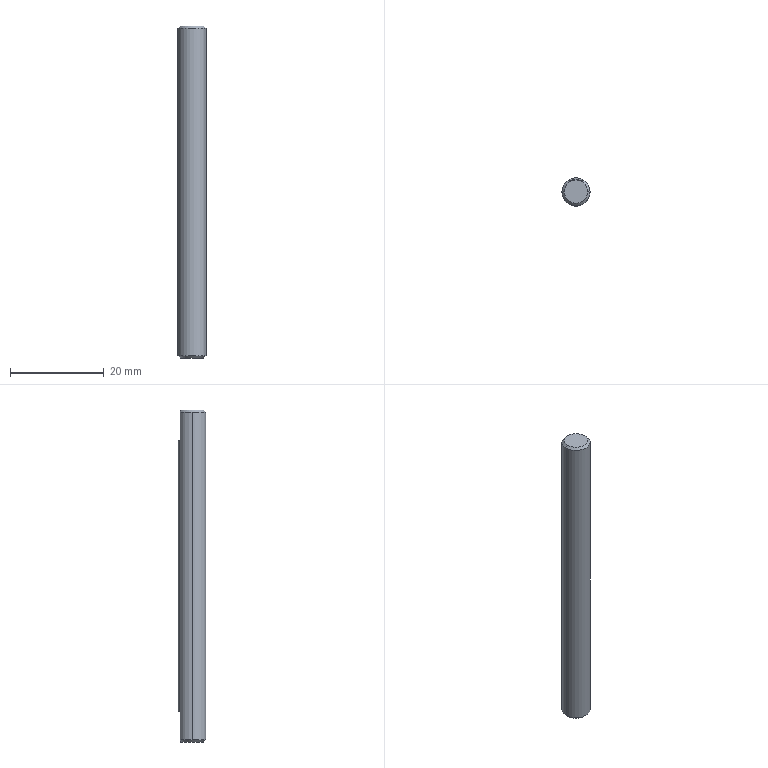Part | STEP file | 10000020485swp000-1 | 1 solid | 14 faces | box 6 x 6 x 71 mm | volume 1989 mm3 | cone 6 | plane 6 | cylinder 2 | commonest cylinder face diameters 6 x2
STEP:
#1=CARTESIAN_POINT('',(2.5,0.,0.));
#2=VERTEX_POINT('',#1);
#3=CARTESIAN_POINT('',(0.,2.5,0.));
#4=VERTEX_POINT('',#3);
#5=CARTESIAN_POINT('',(0.,0.,0.));
#6=DIRECTION('',(0.,0.,1.));
#7=DIRECTION('',(1.,0.,0.));
#8=AXIS2_PLACEMENT_3D('',#5,#6,#7);
#9=CIRCLE('',#8,2.5);
#10=EDGE_CURVE('',#2,#4,#9,.T.);
#11=ORIENTED_EDGE('',*,*,#10,.F.);
#12=CARTESIAN_POINT('',(3.,0.,-0.5));
#13=VERTEX_POINT('',#12);
#14=CARTESIAN_POINT('',(2.5,0.,0.));
#15=DIRECTION('',(0.7071,0.,-0.7071));
#16=VECTOR('',#15,1000.);
#17=LINE('',#14,#16);
#18=EDGE_CURVE('',#2,#13,#17,.T.);
#19=ORIENTED_EDGE('',*,*,#18,.T.);
#20=CARTESIAN_POINT('',(1.658,2.5,-0.5));
#21=VERTEX_POINT('',#20);
#22=CARTESIAN_POINT('',(0.,0.,-0.5));
#23=DIRECTION('',(0.,0.,-1.));
#24=DIRECTION('',(1.,0.,0.));
#25=AXIS2_PLACEMENT_3D('',#22,#23,#24);
#26=CIRCLE('',#25,3.);
#27=EDGE_CURVE('',#21,#13,#26,.T.);
#28=ORIENTED_EDGE('',*,*,#27,.F.);
#29=CARTESIAN_POINT('',(0.,2.5,0.));
#30=CARTESIAN_POINT('',(0.294,2.5,0.));
#31=CARTESIAN_POINT('',(0.5798,2.5,-0.05267));
#32=CARTESIAN_POINT('',(1.139,2.5,-0.2346));
#33=CARTESIAN_POINT('',(1.404,2.5,-0.3596));
#34=CARTESIAN_POINT('',(1.658,2.5,-0.5));
#35=B_SPLINE_CURVE_WITH_KNOTS('',3,(#29,#30,#31,#32,#33,#34),.UNSPECIFIED.,.F.,.F.,(4,2,4),(0.003858,0.004729,0.005601),.UNSPECIFIED.);
#36=EDGE_CURVE('',#4,#21,#35,.T.);
#37=ORIENTED_EDGE('',*,*,#36,.F.);
#38=EDGE_LOOP('',(#11,#19,#28,#37));
#39=FACE_OUTER_BOUND('',#38,.T.);
#40=CARTESIAN_POINT('',(0.,0.,0.));
#41=DIRECTION('',(0.,0.,-1.));
#42=DIRECTION('',(-1.,0.,0.));
#43=AXIS2_PLACEMENT_3D('',#40,#41,#42);
#44=CONICAL_SURFACE('',#43,2.5,0.7854);
#45=ADVANCED_FACE('',(#39),#44,.T.);
#46=ORIENTED_EDGE('',*,*,#18,.F.);
#47=CARTESIAN_POINT('',(-2.5,0.,0.));
#48=VERTEX_POINT('',#47);
#49=CARTESIAN_POINT('',(0.,0.,0.));
#50=DIRECTION('',(0.,0.,1.));
#51=DIRECTION('',(1.,0.,0.));
#52=AXIS2_PLACEMENT_3D('',#49,#50,#51);
#53=CIRCLE('',#52,2.5);
#54=EDGE_CURVE('',#48,#2,#53,.T.);
#55=ORIENTED_EDGE('',*,*,#54,.F.);
#56=CARTESIAN_POINT('',(-3.,0.,-0.5));
#57=VERTEX_POINT('',#56);
#58=CARTESIAN_POINT('',(-2.5,0.,0.));
#59=DIRECTION('',(-0.7071,0.,-0.7071));
#60=VECTOR('',#59,1000.);
#61=LINE('',#58,#60);
#62=EDGE_CURVE('',#48,#57,#61,.T.);
#63=ORIENTED_EDGE('',*,*,#62,.T.);
#64=CARTESIAN_POINT('',(0.,0.,-0.5));
#65=DIRECTION('',(0.,0.,-1.));
#66=DIRECTION('',(1.,0.,0.));
#67=AXIS2_PLACEMENT_3D('',#64,#65,#66);
#68=CIRCLE('',#67,3.);
#69=EDGE_CURVE('',#13,#57,#68,.T.);
#70=ORIENTED_EDGE('',*,*,#69,.F.);
#71=EDGE_LOOP('',(#46,#55,#63,#70));
#72=FACE_OUTER_BOUND('',#71,.T.);
#73=CARTESIAN_POINT('',(0.,0.,0.));
#74=DIRECTION('',(0.,0.,-1.));
#75=DIRECTION('',(-1.,0.,0.));
#76=AXIS2_PLACEMENT_3D('',#73,#74,#75);
#77=CONICAL_SURFACE('',#76,2.5,0.7854);
#78=ADVANCED_FACE('',(#72),#77,.T.);
#79=CARTESIAN_POINT('',(-2.5,0.,-71.));
#80=VERTEX_POINT('',#79);
#81=CARTESIAN_POINT('',(0.,2.5,-71.));
#82=VERTEX_POINT('',#81);
#83=CARTESIAN_POINT('',(0.,0.,-71.));
#84=DIRECTION('',(0.,0.,-1.));
#85=DIRECTION('',(1.,0.,0.));
#86=AXIS2_PLACEMENT_3D('',#83,#84,#85);
#87=CIRCLE('',#86,2.5);
#88=EDGE_CURVE('',#80,#82,#87,.T.);
#89=ORIENTED_EDGE('',*,*,#88,.F.);
#90=CARTESIAN_POINT('',(-3.,0.,-70.5));
#91=VERTEX_POINT('',#90);
#92=CARTESIAN_POINT('',(-3.,0.,-70.5));
#93=DIRECTION('',(-0.7071,0.,0.7071));
#94=VECTOR('',#93,1000.);
#95=LINE('',#92,#94);
#96=EDGE_CURVE('',#80,#91,#95,.T.);
#97=ORIENTED_EDGE('',*,*,#96,.T.);
#98=CARTESIAN_POINT('',(-1.658,2.5,-70.5));
#99=VERTEX_POINT('',#98);
#100=CARTESIAN_POINT('',(0.,0.,-70.5));
#101=DIRECTION('',(0.,0.,1.));
#102=DIRECTION('',(1.,0.,0.));
#103=AXIS2_PLACEMENT_3D('',#100,#101,#102);
#104=CIRCLE('',#103,3.);
#105=EDGE_CURVE('',#99,#91,#104,.T.);
#106=ORIENTED_EDGE('',*,*,#105,.F.);
#107=CARTESIAN_POINT('',(-1.658,2.5,-70.5));
#108=CARTESIAN_POINT('',(-1.404,2.5,-70.641));
#109=CARTESIAN_POINT('',(-1.136,2.5,-70.767));
#110=CARTESIAN_POINT('',(-0.7215,2.5,-70.901));
#111=CARTESIAN_POINT('',(-0.5811,2.5,-70.937));
#112=CARTESIAN_POINT('',(-0.2945,2.5,-70.987));
#113=CARTESIAN_POINT('',(-0.1467,2.5,-71.));
#114=CARTESIAN_POINT('',(0.,2.5,-71.));
#115=B_SPLINE_CURVE_WITH_KNOTS('',3,(#107,#108,#109,#110,#111,#112,#113,#114),.UNSPECIFIED.,.F.,.F.,(4,2,2,4),(0.00212,0.002989,0.003423,0.003858),.UNSPECIFIED.);
#116=EDGE_CURVE('',#99,#82,#115,.T.);
#117=ORIENTED_EDGE('',*,*,#116,.T.);
#118=EDGE_LOOP('',(#89,#97,#106,#117));
#119=FACE_OUTER_BOUND('',#118,.T.);
#120=CARTESIAN_POINT('',(0.,0.,-70.5));
#121=DIRECTION('',(0.,0.,1.));
#122=DIRECTION('',(1.,0.,0.));
#123=AXIS2_PLACEMENT_3D('',#120,#121,#122);
#124=CONICAL_SURFACE('',#123,3.,0.7854);
#125=ADVANCED_FACE('',(#119),#124,.T.);
#126=ORIENTED_EDGE('',*,*,#96,.F.);
#127=CARTESIAN_POINT('',(2.5,0.,-71.));
#128=VERTEX_POINT('',#127);
#129=CARTESIAN_POINT('',(0.,0.,-71.));
#130=DIRECTION('',(0.,0.,-1.));
#131=DIRECTION('',(1.,0.,0.));
#132=AXIS2_PLACEMENT_3D('',#129,#130,#131);
#133=CIRCLE('',#132,2.5);
#134=EDGE_CURVE('',#128,#80,#133,.T.);
#135=ORIENTED_EDGE('',*,*,#134,.F.);
#136=CARTESIAN_POINT('',(3.,0.,-70.5));
#137=VERTEX_POINT('',#136);
#138=CARTESIAN_POINT('',(3.,0.,-70.5));
#139=DIRECTION('',(0.7071,0.,0.7071));
#140=VECTOR('',#139,1000.);
#141=LINE('',#138,#140);
#142=EDGE_CURVE('',#128,#137,#141,.T.);
#143=ORIENTED_EDGE('',*,*,#142,.T.);
#144=CARTESIAN_POINT('',(0.,0.,-70.5));
#145=DIRECTION('',(0.,0.,1.));
#146=DIRECTION('',(1.,0.,0.));
#147=AXIS2_PLACEMENT_3D('',#144,#145,#146);
#148=CIRCLE('',#147,3.);
#149=EDGE_CURVE('',#91,#137,#148,.T.);
#150=ORIENTED_EDGE('',*,*,#149,.F.);
#151=EDGE_LOOP('',(#126,#135,#143,#150));
#152=FACE_OUTER_BOUND('',#151,.T.);
#153=CARTESIAN_POINT('',(0.,0.,-70.5));
#154=DIRECTION('',(0.,0.,1.));
#155=DIRECTION('',(1.,0.,0.));
#156=AXIS2_PLACEMENT_3D('',#153,#154,#155);
#157=CONICAL_SURFACE('',#156,3.,0.7854);
#158=ADVANCED_FACE('',(#152),#157,.T.);
#159=ORIENTED_EDGE('',*,*,#105,.T.);
#160=CARTESIAN_POINT('',(-3.,0.,-71.));
#161=DIRECTION('',(0.,0.,1.));
#162=VECTOR('',#161,1000.);
#163=LINE('',#160,#162);
#164=EDGE_CURVE('',#91,#57,#163,.T.);
#165=ORIENTED_EDGE('',*,*,#164,.T.);
#166=CARTESIAN_POINT('',(-1.658,2.5,-0.5));
#167=VERTEX_POINT('',#166);
#168=CARTESIAN_POINT('',(0.,0.,-0.5));
#169=DIRECTION('',(0.,0.,-1.));
#170=DIRECTION('',(1.,0.,0.));
#171=AXIS2_PLACEMENT_3D('',#168,#169,#170);
#172=CIRCLE('',#171,3.);
#173=EDGE_CURVE('',#57,#167,#172,.T.);
#174=ORIENTED_EDGE('',*,*,#173,.T.);
#175=CARTESIAN_POINT('',(-1.658,2.5,-6.5));
#176=VERTEX_POINT('',#175);
#177=CARTESIAN_POINT('',(-1.658,2.5,-6.5));
#178=DIRECTION('',(0.,0.,1.));
#179=VECTOR('',#178,1000.);
#180=LINE('',#177,#179);
#181=EDGE_CURVE('',#176,#167,#180,.T.);
#182=ORIENTED_EDGE('',*,*,#181,.F.);
#183=CARTESIAN_POINT('',(1.658,2.5,-6.5));
#184=VERTEX_POINT('',#183);
#185=CARTESIAN_POINT('',(0.,0.,-6.5));
#186=DIRECTION('',(0.,0.,1.));
#187=DIRECTION('',(1.,0.,0.));
#188=AXIS2_PLACEMENT_3D('',#185,#186,#187);
#189=CIRCLE('',#188,3.);
#190=EDGE_CURVE('',#184,#176,#189,.T.);
#191=ORIENTED_EDGE('',*,*,#190,.F.);
#192=CARTESIAN_POINT('',(1.658,2.5,-6.5));
#193=DIRECTION('',(0.,0.,1.));
#194=VECTOR('',#193,1000.);
#195=LINE('',#192,#194);
#196=EDGE_CURVE('',#184,#21,#195,.T.);
#197=ORIENTED_EDGE('',*,*,#196,.T.);
#198=ORIENTED_EDGE('',*,*,#27,.T.);
#199=CARTESIAN_POINT('',(3.,0.,-71.));
#200=DIRECTION('',(0.,0.,1.));
#201=VECTOR('',#200,1000.);
#202=LINE('',#199,#201);
#203=EDGE_CURVE('',#137,#13,#202,.T.);
#204=ORIENTED_EDGE('',*,*,#203,.F.);
#205=CARTESIAN_POINT('',(1.658,2.5,-70.5));
#206=VERTEX_POINT('',#205);
#207=CARTESIAN_POINT('',(0.,0.,-70.5));
#208=DIRECTION('',(0.,0.,1.));
#209=DIRECTION('',(1.,0.,0.));
#210=AXIS2_PLACEMENT_3D('',#207,#208,#209);
#211=CIRCLE('',#210,3.);
#212=EDGE_CURVE('',#137,#206,#211,.T.);
#213=ORIENTED_EDGE('',*,*,#212,.T.);
#214=CARTESIAN_POINT('',(1.658,2.5,-64.5));
#215=VERTEX_POINT('',#214);
#216=CARTESIAN_POINT('',(1.658,2.5,-64.5));
#217=DIRECTION('',(0.,0.,-1.));
#218=VECTOR('',#217,1000.);
#219=LINE('',#216,#218);
#220=EDGE_CURVE('',#215,#206,#219,.T.);
#221=ORIENTED_EDGE('',*,*,#220,.F.);
#222=CARTESIAN_POINT('',(-1.658,2.5,-64.5));
#223=VERTEX_POINT('',#222);
#224=CARTESIAN_POINT('',(0.,0.,-64.5));
#225=DIRECTION('',(0.,0.,1.));
#226=DIRECTION('',(1.,0.,0.));
#227=AXIS2_PLACEMENT_3D('',#224,#225,#226);
#228=CIRCLE('',#227,3.);
#229=EDGE_CURVE('',#215,#223,#228,.T.);
#230=ORIENTED_EDGE('',*,*,#229,.T.);
#231=CARTESIAN_POINT('',(-1.658,2.5,-64.5));
#232=DIRECTION('',(0.,0.,-1.));
#233=VECTOR('',#232,1000.);
#234=LINE('',#231,#233);
#235=EDGE_CURVE('',#223,#99,#234,.T.);
#236=ORIENTED_EDGE('',*,*,#235,.T.);
#237=EDGE_LOOP('',(#159,#165,#174,#182,#191,#197,#198,#204,#213,#221,#230,#236));
#238=FACE_OUTER_BOUND('',#237,.T.);
#239=CARTESIAN_POINT('',(0.,0.,-71.));
#240=DIRECTION('',(0.,0.,1.));
#241=DIRECTION('',(1.,0.,0.));
#242=AXIS2_PLACEMENT_3D('',#239,#240,#241);
#243=CYLINDRICAL_SURFACE('',#242,3.);
#244=ADVANCED_FACE('',(#238),#243,.T.);
#245=ORIENTED_EDGE('',*,*,#164,.F.);
#246=ORIENTED_EDGE('',*,*,#149,.T.);
#247=ORIENTED_EDGE('',*,*,#203,.T.);
#248=ORIENTED_EDGE('',*,*,#69,.T.);
#249=EDGE_LOOP('',(#245,#246,#247,#248));
#250=FACE_OUTER_BOUND('',#249,.T.);
#251=CARTESIAN_POINT('',(0.,0.,-71.));
#252=DIRECTION('',(0.,0.,1.));
#253=DIRECTION('',(1.,0.,0.));
#254=AXIS2_PLACEMENT_3D('',#251,#252,#253);
#255=CYLINDRICAL_SURFACE('',#254,3.);
#256=ADVANCED_FACE('',(#250),#255,.T.);
#257=ORIENTED_EDGE('',*,*,#142,.F.);
#258=CARTESIAN_POINT('',(0.,0.,-71.));
#259=DIRECTION('',(0.,0.,-1.));
#260=DIRECTION('',(1.,0.,0.));
#261=AXIS2_PLACEMENT_3D('',#258,#259,#260);
#262=CIRCLE('',#261,2.5);
#263=EDGE_CURVE('',#82,#128,#262,.T.);
#264=ORIENTED_EDGE('',*,*,#263,.F.);
#265=CARTESIAN_POINT('',(0.,2.5,-71.));
#266=CARTESIAN_POINT('',(0.294,2.5,-71.));
#267=CARTESIAN_POINT('',(0.5798,2.5,-70.947));
#268=CARTESIAN_POINT('',(1.139,2.5,-70.765));
#269=CARTESIAN_POINT('',(1.404,2.5,-70.64));
#270=CARTESIAN_POINT('',(1.658,2.5,-70.5));
#271=B_SPLINE_CURVE_WITH_KNOTS('',3,(#265,#266,#267,#268,#269,#270),.UNSPECIFIED.,.F.,.F.,(4,2,4),(0.003858,0.004729,0.005601),.UNSPECIFIED.);
#272=EDGE_CURVE('',#82,#206,#271,.T.);
#273=ORIENTED_EDGE('',*,*,#272,.T.);
#274=ORIENTED_EDGE('',*,*,#212,.F.);
#275=EDGE_LOOP('',(#257,#264,#273,#274));
#276=FACE_OUTER_BOUND('',#275,.T.);
#277=CARTESIAN_POINT('',(0.,0.,-70.5));
#278=DIRECTION('',(0.,0.,1.));
#279=DIRECTION('',(1.,0.,0.));
#280=AXIS2_PLACEMENT_3D('',#277,#278,#279);
#281=CONICAL_SURFACE('',#280,3.,0.7854);
#282=ADVANCED_FACE('',(#276),#281,.T.);
#283=ORIENTED_EDGE('',*,*,#263,.T.);
#284=ORIENTED_EDGE('',*,*,#134,.T.);
#285=ORIENTED_EDGE('',*,*,#88,.T.);
#286=EDGE_LOOP('',(#283,#284,#285));
#287=FACE_OUTER_BOUND('',#286,.T.);
#288=CARTESIAN_POINT('',(0.,0.,-71.));
#289=DIRECTION('',(0.,0.,1.));
#290=DIRECTION('',(1.,0.,0.));
#291=AXIS2_PLACEMENT_3D('',#288,#289,#290);
#292=PLANE('',#291);
#293=ADVANCED_FACE('',(#287),#292,.F.);
#294=CARTESIAN_POINT('',(0.,0.,0.));
#295=DIRECTION('',(0.,0.,1.));
#296=DIRECTION('',(1.,0.,0.));
#297=AXIS2_PLACEMENT_3D('',#294,#295,#296);
#298=CIRCLE('',#297,2.5);
#299=EDGE_CURVE('',#4,#48,#298,.T.);
#300=ORIENTED_EDGE('',*,*,#299,.T.);
#301=ORIENTED_EDGE('',*,*,#54,.T.);
#302=ORIENTED_EDGE('',*,*,#10,.T.);
#303=EDGE_LOOP('',(#300,#301,#302));
#304=FACE_OUTER_BOUND('',#303,.T.);
#305=CARTESIAN_POINT('',(0.,0.,0.));
#306=DIRECTION('',(0.,0.,1.));
#307=DIRECTION('',(1.,0.,0.));
#308=AXIS2_PLACEMENT_3D('',#305,#306,#307);
#309=PLANE('',#308);
#310=ADVANCED_FACE('',(#304),#309,.T.);
#311=ORIENTED_EDGE('',*,*,#62,.F.);
#312=ORIENTED_EDGE('',*,*,#299,.F.);
#313=CARTESIAN_POINT('',(-1.658,2.5,-0.5));
#314=CARTESIAN_POINT('',(-1.404,2.5,-0.3594));
#315=CARTESIAN_POINT('',(-1.136,2.5,-0.2335));
#316=CARTESIAN_POINT('',(-0.7215,2.5,-0.09874));
#317=CARTESIAN_POINT('',(-0.5811,2.5,-0.06276));
#318=CARTESIAN_POINT('',(-0.2945,2.5,-0.01333));
#319=CARTESIAN_POINT('',(-0.1467,2.5,0.));
#320=CARTESIAN_POINT('',(0.,2.5,0.));
#321=B_SPLINE_CURVE_WITH_KNOTS('',3,(#313,#314,#315,#316,#317,#318,#319,#320),.UNSPECIFIED.,.F.,.F.,(4,2,2,4),(0.00212,0.002989,0.003423,0.003858),.UNSPECIFIED.);
#322=EDGE_CURVE('',#167,#4,#321,.T.);
#323=ORIENTED_EDGE('',*,*,#322,.F.);
#324=ORIENTED_EDGE('',*,*,#173,.F.);
#325=EDGE_LOOP('',(#311,#312,#323,#324));
#326=FACE_OUTER_BOUND('',#325,.T.);
#327=CARTESIAN_POINT('',(0.,0.,0.));
#328=DIRECTION('',(0.,0.,-1.));
#329=DIRECTION('',(-1.,0.,0.));
#330=AXIS2_PLACEMENT_3D('',#327,#328,#329);
#331=CONICAL_SURFACE('',#330,2.5,0.7854);
#332=ADVANCED_FACE('',(#326),#331,.T.);
#333=ORIENTED_EDGE('',*,*,#322,.T.);
#334=ORIENTED_EDGE('',*,*,#36,.T.);
#335=ORIENTED_EDGE('',*,*,#196,.F.);
#336=CARTESIAN_POINT('',(1.658,2.5,-6.5));
#337=DIRECTION('',(1.,0.,0.));
#338=VECTOR('',#337,1000.);
#339=LINE('',#336,#338);
#340=EDGE_CURVE('',#176,#184,#339,.T.);
#341=ORIENTED_EDGE('',*,*,#340,.F.);
#342=ORIENTED_EDGE('',*,*,#181,.T.);
#343=EDGE_LOOP('',(#333,#334,#335,#341,#342));
#344=FACE_OUTER_BOUND('',#343,.T.);
#345=CARTESIAN_POINT('',(1.658,2.5,-6.5));
#346=DIRECTION('',(0.,-1.,0.));
#347=DIRECTION('',(0.,0.,-1.));
#348=AXIS2_PLACEMENT_3D('',#345,#346,#347);
#349=PLANE('',#348);
#350=ADVANCED_FACE('',(#344),#349,.F.);
#351=ORIENTED_EDGE('',*,*,#190,.T.);
#352=ORIENTED_EDGE('',*,*,#340,.T.);
#353=EDGE_LOOP('',(#351,#352));
#354=FACE_OUTER_BOUND('',#353,.T.);
#355=CARTESIAN_POINT('',(0.,0.,-6.5));
#356=DIRECTION('',(0.,0.,1.));
#357=DIRECTION('',(1.,0.,0.));
#358=AXIS2_PLACEMENT_3D('',#355,#356,#357);
#359=PLANE('',#358);
#360=ADVANCED_FACE('',(#354),#359,.T.);
#361=ORIENTED_EDGE('',*,*,#235,.F.);
#362=CARTESIAN_POINT('',(1.658,2.5,-64.5));
#363=DIRECTION('',(1.,0.,0.));
#364=VECTOR('',#363,1000.);
#365=LINE('',#362,#364);
#366=EDGE_CURVE('',#223,#215,#365,.T.);
#367=ORIENTED_EDGE('',*,*,#366,.T.);
#368=ORIENTED_EDGE('',*,*,#220,.T.);
#369=ORIENTED_EDGE('',*,*,#272,.F.);
#370=ORIENTED_EDGE('',*,*,#116,.F.);
#371=EDGE_LOOP('',(#361,#367,#368,#369,#370));
#372=FACE_OUTER_BOUND('',#371,.T.);
#373=CARTESIAN_POINT('',(1.658,2.5,-64.5));
#374=DIRECTION('',(0.,1.,0.));
#375=DIRECTION('',(0.,0.,1.));
#376=AXIS2_PLACEMENT_3D('',#373,#374,#375);
#377=PLANE('',#376);
#378=ADVANCED_FACE('',(#372),#377,.T.);
#379=ORIENTED_EDGE('',*,*,#229,.F.);
#380=ORIENTED_EDGE('',*,*,#366,.F.);
#381=EDGE_LOOP('',(#379,#380));
#382=FACE_OUTER_BOUND('',#381,.T.);
#383=CARTESIAN_POINT('',(0.,0.,-64.5));
#384=DIRECTION('',(0.,0.,-1.));
#385=DIRECTION('',(1.,0.,0.));
#386=AXIS2_PLACEMENT_3D('',#383,#384,#385);
#387=PLANE('',#386);
#388=ADVANCED_FACE('',(#382),#387,.T.);
#389=CLOSED_SHELL('',(#45,#78,#125,#158,#244,#256,#282,#293,#310,#332,#350,#360,#378,#388));
#390=MANIFOLD_SOLID_BREP('',#389);
#391=CARTESIAN_POINT('',(0.,0.,0.));
#392=DIRECTION('',(0.,0.,1.));
#393=DIRECTION('',(1.,0.,0.));
#394=AXIS2_PLACEMENT_3D('',#391,#392,#393);
#395=(LENGTH_UNIT()NAMED_UNIT(*)SI_UNIT(.MILLI.,.METRE.));
#396=UNCERTAINTY_MEASURE_WITH_UNIT(LENGTH_MEASURE(0.00001),#395,'','');
#397=(NAMED_UNIT(*)PLANE_ANGLE_UNIT()SI_UNIT($,.RADIAN.));
#398=(NAMED_UNIT(*)SI_UNIT($,.STERADIAN.)SOLID_ANGLE_UNIT());
#399=(GEOMETRIC_REPRESENTATION_CONTEXT(3)GLOBAL_UNCERTAINTY_ASSIGNED_CONTEXT((#396))GLOBAL_UNIT_ASSIGNED_CONTEXT((#395,#397,#398))REPRESENTATION_CONTEXT('',''));
#400=ADVANCED_BREP_SHAPE_REPRESENTATION('',(#390,#394),#399);